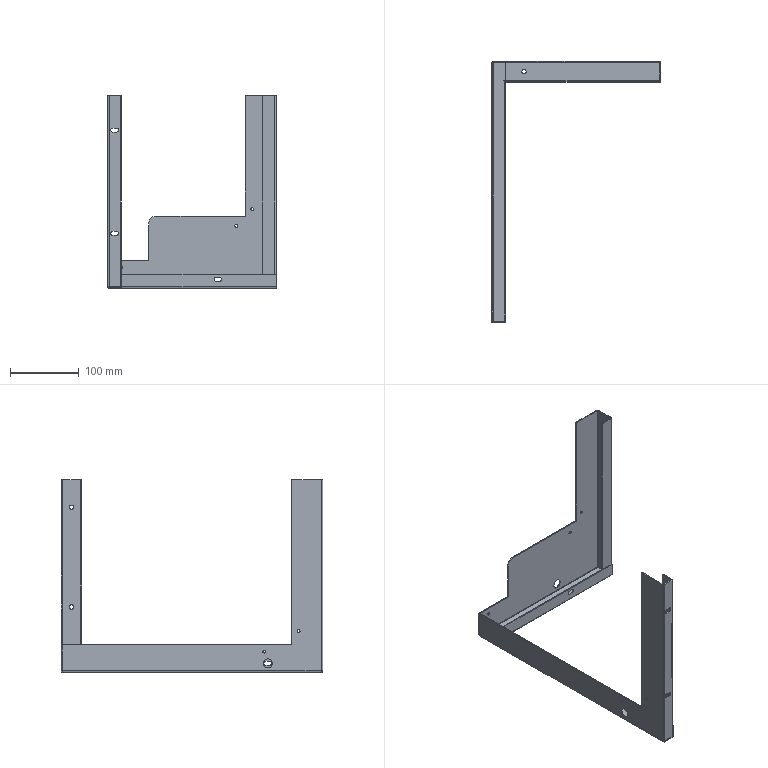Part | SolidWorks | features ICE 15, SMMiteredFlange 7, LPattern 2, Cut 1, EdgeFlange 1, Fillet 1, FlatPattern 1, SMBaseFlange 1, SheetMetal 1 | 1 solid | 138 faces | box 245 x 380 x 280 mm | volume 150537 mm3 | plane 90 | cylinder 48 | commonest cylinder face diameters 4 x17 1 x9 6 x9 6.4 x6 13 x4 4.415 x2